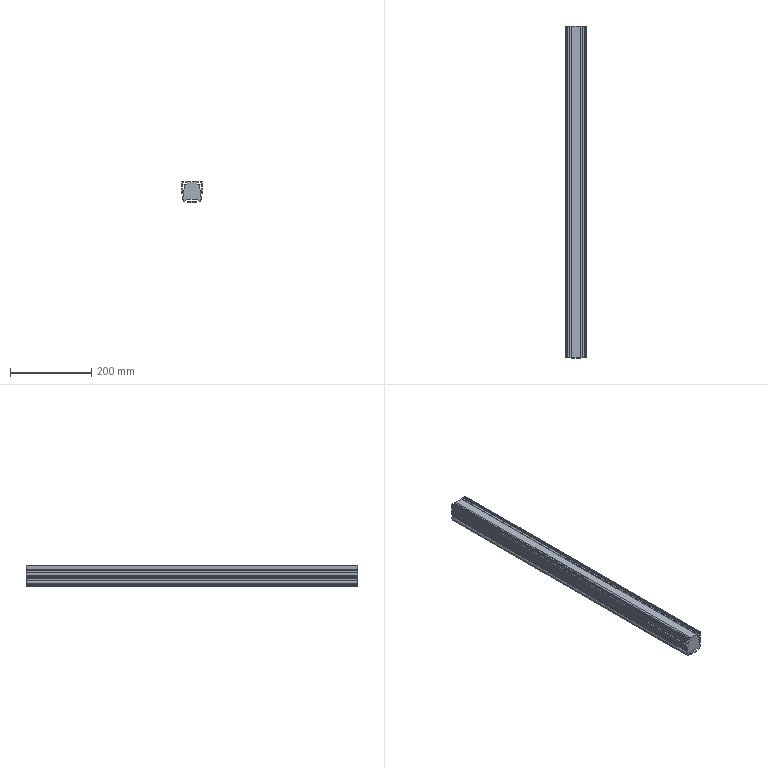Part | STEP file | Copy of 50-2016 profile^K50A-1H20-S(formula driven)-L700-motor left- | 2 solids | 143 faces | box 50 x 815 x 52.45 mm | volume 1652118 mm3 | plane 72 | cylinder 71 | commonest cylinder face diameters 0.4 x58 4.2 x6 4 x5 8 x2